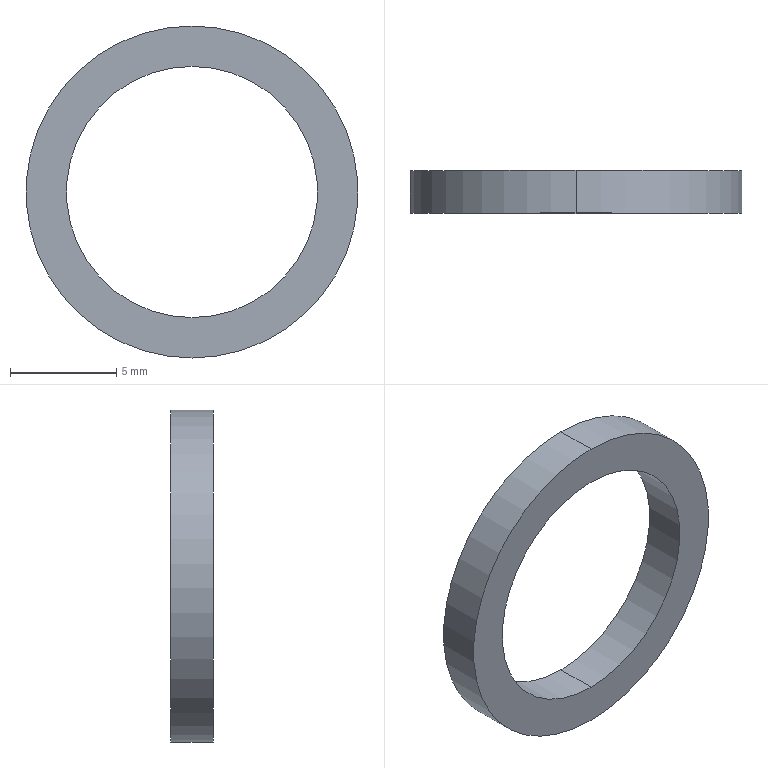Part | SolidWorks | features Extrusion 1 | 1 solid | 6 faces | box 15.6 x 2 x 15.6 mm | volume 163.551 mm3 | cylinder 4 | plane 2 | commonest cylinder face diameters 11.8 x2 15.6 x2
STEP:
#1=CARTESIAN_POINT('',(0.,2.,-5.9));
#2=VERTEX_POINT('',#1);
#3=CARTESIAN_POINT('',(0.,2.,5.9));
#4=VERTEX_POINT('',#3);
#5=CARTESIAN_POINT('',(0.,2.,0.));
#6=DIRECTION('',(0.,1.,0.));
#7=DIRECTION('',(0.,0.,1.));
#8=AXIS2_PLACEMENT_3D('',#5,#6,#7);
#9=CIRCLE('',#8,5.9);
#10=EDGE_CURVE('',#2,#4,#9,.T.);
#11=ORIENTED_EDGE('',*,*,#10,.T.);
#12=CARTESIAN_POINT('',(0.,0.,5.9));
#13=VERTEX_POINT('',#12);
#14=CARTESIAN_POINT('',(0.,2.,5.9));
#15=DIRECTION('',(0.,-1.,0.));
#16=VECTOR('',#15,1000.);
#17=LINE('',#14,#16);
#18=EDGE_CURVE('',#4,#13,#17,.T.);
#19=ORIENTED_EDGE('',*,*,#18,.T.);
#20=CARTESIAN_POINT('',(0.,0.,-5.9));
#21=VERTEX_POINT('',#20);
#22=CARTESIAN_POINT('',(0.,0.,0.));
#23=DIRECTION('',(0.,1.,0.));
#24=DIRECTION('',(0.,0.,1.));
#25=AXIS2_PLACEMENT_3D('',#22,#23,#24);
#26=CIRCLE('',#25,5.9);
#27=EDGE_CURVE('',#21,#13,#26,.T.);
#28=ORIENTED_EDGE('',*,*,#27,.F.);
#29=CARTESIAN_POINT('',(0.,2.,-5.9));
#30=DIRECTION('',(0.,-1.,0.));
#31=VECTOR('',#30,1000.);
#32=LINE('',#29,#31);
#33=EDGE_CURVE('',#2,#21,#32,.T.);
#34=ORIENTED_EDGE('',*,*,#33,.F.);
#35=EDGE_LOOP('',(#11,#19,#28,#34));
#36=FACE_OUTER_BOUND('',#35,.T.);
#37=CARTESIAN_POINT('',(0.,2.,0.));
#38=DIRECTION('',(0.,-1.,0.));
#39=DIRECTION('',(0.,0.,-1.));
#40=AXIS2_PLACEMENT_3D('',#37,#38,#39);
#41=CYLINDRICAL_SURFACE('',#40,5.9);
#42=ADVANCED_FACE('',(#36),#41,.F.);
#43=CARTESIAN_POINT('',(0.,2.,7.8));
#44=VERTEX_POINT('',#43);
#45=CARTESIAN_POINT('',(0.,2.,-7.8));
#46=VERTEX_POINT('',#45);
#47=CARTESIAN_POINT('',(0.,2.,0.));
#48=DIRECTION('',(0.,1.,0.));
#49=DIRECTION('',(0.,0.,1.));
#50=AXIS2_PLACEMENT_3D('',#47,#48,#49);
#51=CIRCLE('',#50,7.8);
#52=EDGE_CURVE('',#44,#46,#51,.T.);
#53=ORIENTED_EDGE('',*,*,#52,.F.);
#54=CARTESIAN_POINT('',(0.,0.,7.8));
#55=VERTEX_POINT('',#54);
#56=CARTESIAN_POINT('',(0.,2.,7.8));
#57=DIRECTION('',(0.,-1.,0.));
#58=VECTOR('',#57,1000.);
#59=LINE('',#56,#58);
#60=EDGE_CURVE('',#44,#55,#59,.T.);
#61=ORIENTED_EDGE('',*,*,#60,.T.);
#62=CARTESIAN_POINT('',(0.,0.,-7.8));
#63=VERTEX_POINT('',#62);
#64=CARTESIAN_POINT('',(0.,0.,0.));
#65=DIRECTION('',(0.,1.,0.));
#66=DIRECTION('',(0.,0.,1.));
#67=AXIS2_PLACEMENT_3D('',#64,#65,#66);
#68=CIRCLE('',#67,7.8);
#69=EDGE_CURVE('',#55,#63,#68,.T.);
#70=ORIENTED_EDGE('',*,*,#69,.T.);
#71=CARTESIAN_POINT('',(0.,2.,-7.8));
#72=DIRECTION('',(0.,-1.,0.));
#73=VECTOR('',#72,1000.);
#74=LINE('',#71,#73);
#75=EDGE_CURVE('',#46,#63,#74,.T.);
#76=ORIENTED_EDGE('',*,*,#75,.F.);
#77=EDGE_LOOP('',(#53,#61,#70,#76));
#78=FACE_OUTER_BOUND('',#77,.T.);
#79=CARTESIAN_POINT('',(0.,2.,0.));
#80=DIRECTION('',(0.,-1.,0.));
#81=DIRECTION('',(0.,0.,-1.));
#82=AXIS2_PLACEMENT_3D('',#79,#80,#81);
#83=CYLINDRICAL_SURFACE('',#82,7.8);
#84=ADVANCED_FACE('',(#78),#83,.T.);
#85=CARTESIAN_POINT('',(0.,2.,0.));
#86=DIRECTION('',(0.,1.,0.));
#87=DIRECTION('',(0.,0.,1.));
#88=AXIS2_PLACEMENT_3D('',#85,#86,#87);
#89=CIRCLE('',#88,7.8);
#90=EDGE_CURVE('',#46,#44,#89,.T.);
#91=ORIENTED_EDGE('',*,*,#90,.T.);
#92=ORIENTED_EDGE('',*,*,#52,.T.);
#93=EDGE_LOOP('',(#91,#92));
#94=FACE_OUTER_BOUND('',#93,.T.);
#95=ORIENTED_EDGE('',*,*,#10,.F.);
#96=CARTESIAN_POINT('',(0.,2.,0.));
#97=DIRECTION('',(0.,1.,0.));
#98=DIRECTION('',(0.,0.,1.));
#99=AXIS2_PLACEMENT_3D('',#96,#97,#98);
#100=CIRCLE('',#99,5.9);
#101=EDGE_CURVE('',#4,#2,#100,.T.);
#102=ORIENTED_EDGE('',*,*,#101,.F.);
#103=EDGE_LOOP('',(#95,#102));
#104=FACE_BOUND('',#103,.T.);
#105=CARTESIAN_POINT('',(0.,2.,0.));
#106=DIRECTION('',(0.,1.,0.));
#107=DIRECTION('',(0.,0.,1.));
#108=AXIS2_PLACEMENT_3D('',#105,#106,#107);
#109=PLANE('',#108);
#110=ADVANCED_FACE('',(#94,#104),#109,.T.);
#111=CARTESIAN_POINT('',(0.,0.,0.));
#112=DIRECTION('',(0.,1.,0.));
#113=DIRECTION('',(0.,0.,1.));
#114=AXIS2_PLACEMENT_3D('',#111,#112,#113);
#115=CIRCLE('',#114,7.8);
#116=EDGE_CURVE('',#63,#55,#115,.T.);
#117=ORIENTED_EDGE('',*,*,#116,.F.);
#118=ORIENTED_EDGE('',*,*,#69,.F.);
#119=EDGE_LOOP('',(#117,#118));
#120=FACE_OUTER_BOUND('',#119,.T.);
#121=ORIENTED_EDGE('',*,*,#27,.T.);
#122=CARTESIAN_POINT('',(0.,0.,0.));
#123=DIRECTION('',(0.,1.,0.));
#124=DIRECTION('',(0.,0.,1.));
#125=AXIS2_PLACEMENT_3D('',#122,#123,#124);
#126=CIRCLE('',#125,5.9);
#127=EDGE_CURVE('',#13,#21,#126,.T.);
#128=ORIENTED_EDGE('',*,*,#127,.T.);
#129=EDGE_LOOP('',(#121,#128));
#130=FACE_BOUND('',#129,.T.);
#131=CARTESIAN_POINT('',(0.,0.,0.));
#132=DIRECTION('',(0.,1.,0.));
#133=DIRECTION('',(0.,0.,1.));
#134=AXIS2_PLACEMENT_3D('',#131,#132,#133);
#135=PLANE('',#134);
#136=ADVANCED_FACE('',(#120,#130),#135,.F.);
#137=ORIENTED_EDGE('',*,*,#60,.F.);
#138=ORIENTED_EDGE('',*,*,#90,.F.);
#139=ORIENTED_EDGE('',*,*,#75,.T.);
#140=ORIENTED_EDGE('',*,*,#116,.T.);
#141=EDGE_LOOP('',(#137,#138,#139,#140));
#142=FACE_OUTER_BOUND('',#141,.T.);
#143=CARTESIAN_POINT('',(0.,2.,0.));
#144=DIRECTION('',(0.,-1.,0.));
#145=DIRECTION('',(0.,0.,-1.));
#146=AXIS2_PLACEMENT_3D('',#143,#144,#145);
#147=CYLINDRICAL_SURFACE('',#146,7.8);
#148=ADVANCED_FACE('',(#142),#147,.T.);
#149=ORIENTED_EDGE('',*,*,#18,.F.);
#150=ORIENTED_EDGE('',*,*,#101,.T.);
#151=ORIENTED_EDGE('',*,*,#33,.T.);
#152=ORIENTED_EDGE('',*,*,#127,.F.);
#153=EDGE_LOOP('',(#149,#150,#151,#152));
#154=FACE_OUTER_BOUND('',#153,.T.);
#155=CARTESIAN_POINT('',(0.,2.,0.));
#156=DIRECTION('',(0.,-1.,0.));
#157=DIRECTION('',(0.,0.,-1.));
#158=AXIS2_PLACEMENT_3D('',#155,#156,#157);
#159=CYLINDRICAL_SURFACE('',#158,5.9);
#160=ADVANCED_FACE('',(#154),#159,.F.);
#161=CLOSED_SHELL('',(#42,#84,#110,#136,#148,#160));
#162=MANIFOLD_SOLID_BREP('',#161);
#163=CARTESIAN_POINT('',(0.,0.,0.));
#164=DIRECTION('',(0.,0.,1.));
#165=DIRECTION('',(1.,0.,0.));
#166=AXIS2_PLACEMENT_3D('',#163,#164,#165);
#167=(LENGTH_UNIT()NAMED_UNIT(*)SI_UNIT(.MILLI.,.METRE.));
#168=UNCERTAINTY_MEASURE_WITH_UNIT(LENGTH_MEASURE(0.00001),#167,'','');
#169=(NAMED_UNIT(*)PLANE_ANGLE_UNIT()SI_UNIT($,.RADIAN.));
#170=(NAMED_UNIT(*)SI_UNIT($,.STERADIAN.)SOLID_ANGLE_UNIT());
#171=(GEOMETRIC_REPRESENTATION_CONTEXT(3)GLOBAL_UNCERTAINTY_ASSIGNED_CONTEXT((#168))GLOBAL_UNIT_ASSIGNED_CONTEXT((#167,#169,#170))REPRESENTATION_CONTEXT('',''));
#172=ADVANCED_BREP_SHAPE_REPRESENTATION('',(#162,#166),#171);